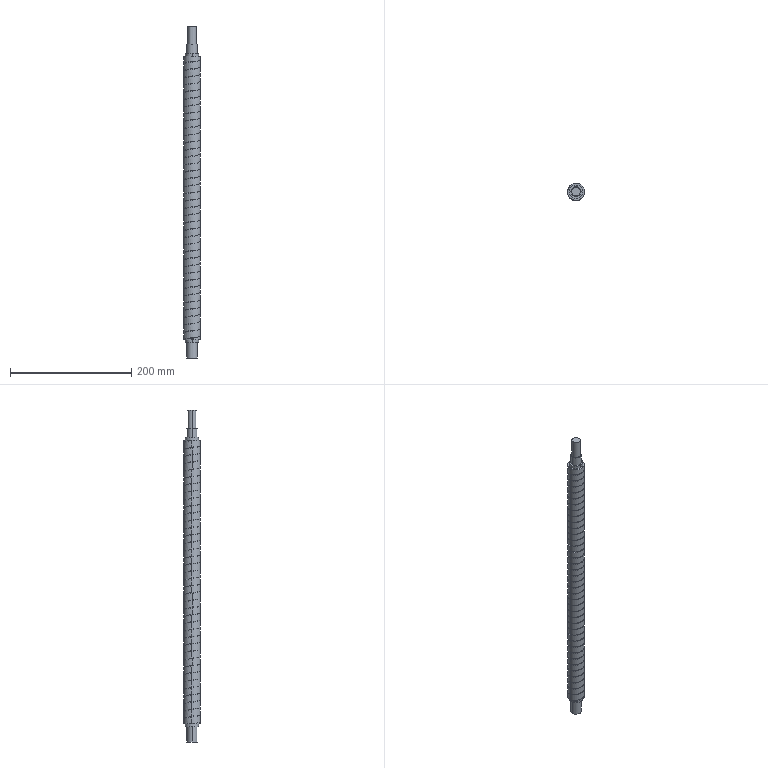Part | SolidWorks | features BaseBody 1 | 1 solid | 98 faces | box 28 x 28 x 548 mm | volume 304343 mm3 | cylinder 90 | plane 7 | spline 1 | commonest cylinder face diameters 28 x80 17 x4 22 x4 14 x2